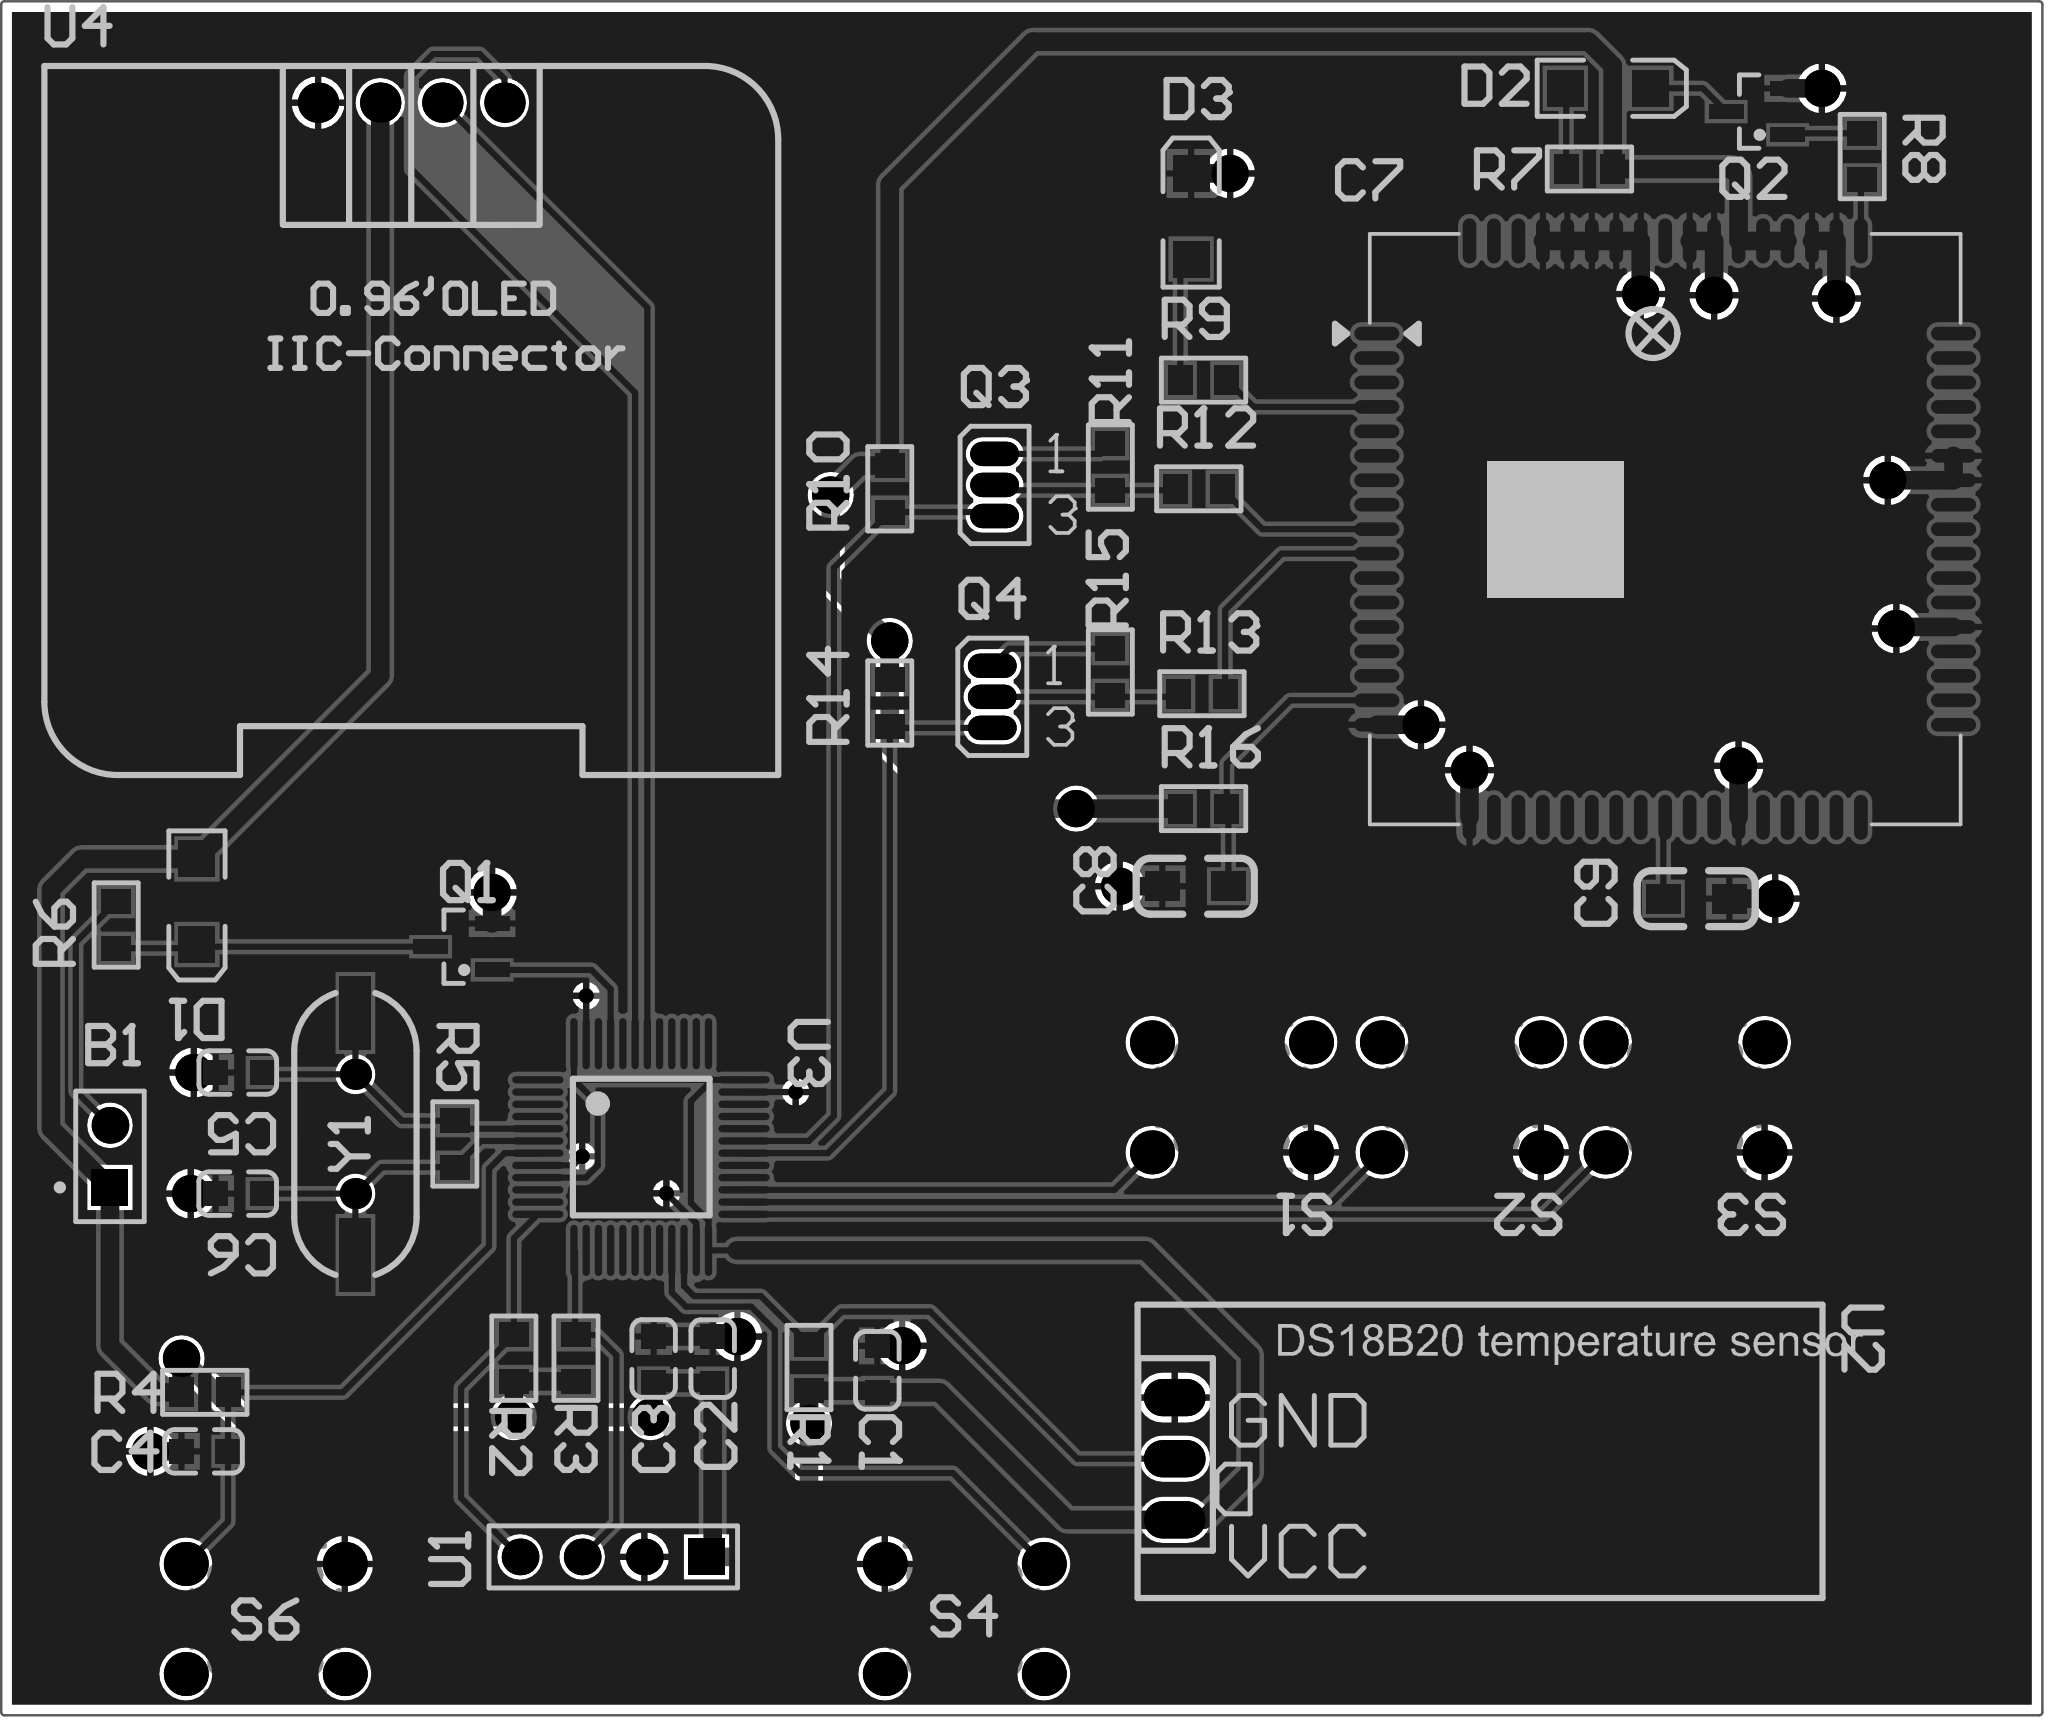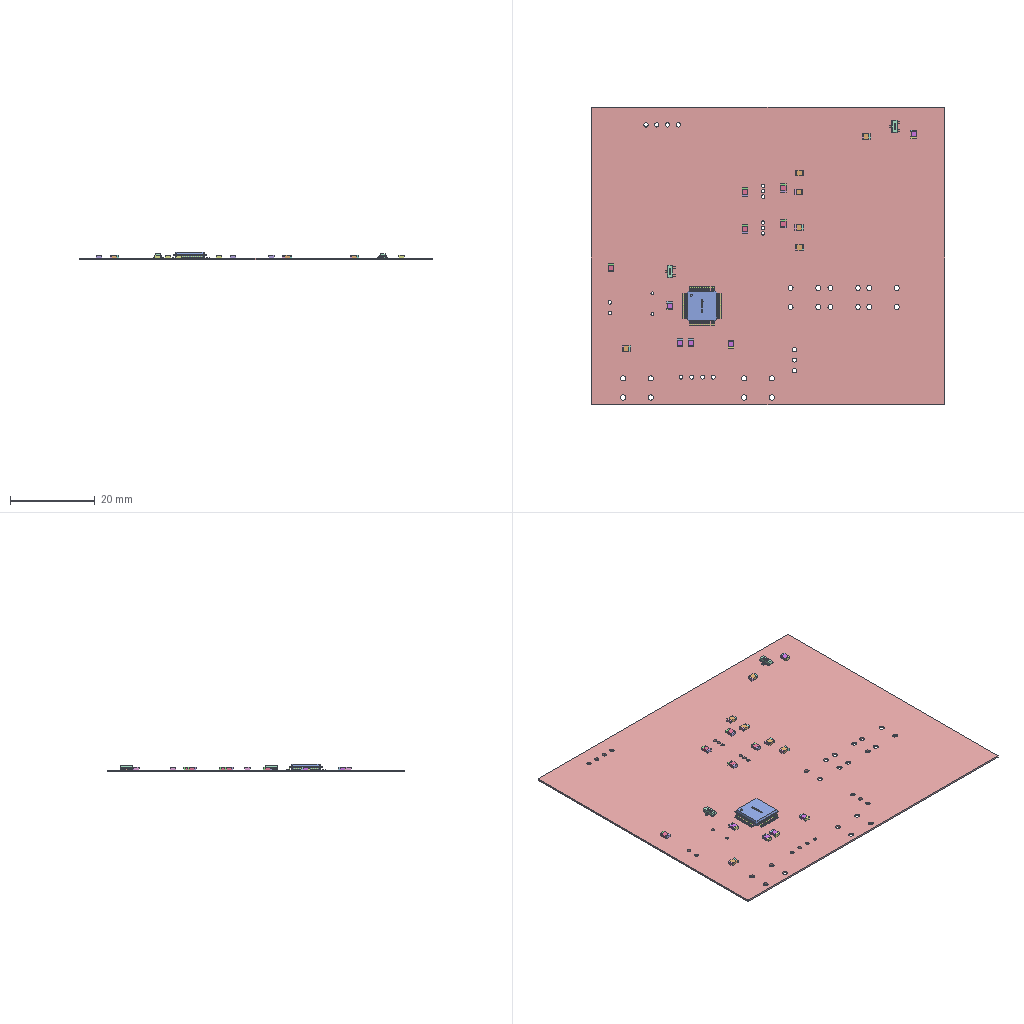Circuit board layout | Altium Designer | box 83.4 x 70.1 x 1.9 mm
Layer stack:
# Altium Designer layer stack of  (unit mm; dielectric type: 0 none, 1 core, 2 prepreg, 3 surface material)
index,name,kind,layer,copper_thickness_mm,dielectric_type,dielectric_thickness_mm,dielectric_material,dielectric_constant
0,Top Paste,other,,,,,,
1,Top Overlay,other,,,,,,
2,Top Solder,dielectric,,,3,0.0102,Solder Resist,3.5
3,Top Layer,copper,Top Layer,0.0356,,,,
4,Dielectric 1,dielectric,,,0,0.32,FR-4,4.8
5,Bottom Layer,copper,Bottom Layer,0.0356,,,,
6,Bottom Solder,dielectric,,,3,0.0102,Solder Resist,3.5
7,Bottom Overlay,other,,,,,,
8,Bottom Paste,other,,,,,,
# drill layer pairs: low layer,high layer
drill_pair,Top Layer,Bottom Layer
Part placement:
Designator,Comment,Layer,Footprint,Center-X(mm),Center-Y(mm),Rotation
Y1,XTAL,TopLayer,XTAL_US,53.086,49.049,90
U4,OLED display,TopLayer,0.96OLED_4P,55.371,91.231,360
U3,STM32,TopLayer,LQFP48_7X7,64.757,48.514,270
U2,DS18B20 temperature sensor,TopLayer,DS18B20,86.58,35.766,360
U1,ASR01 speech recognition module,TopLayer,HDR1X4,63.627,31.75,180
S6,Key,TopLayer,四脚轻触开关,49.403,29.21,0
S4,Value increase key,TopLayer,四脚轻触开关,77.978,29.21,0
S3,Value decrease key,TopLayer,四脚轻触开关,107.442,50.546,180
S2,Cursor switch key,TopLayer,四脚轻触开关,98.298,50.546,180
S1,Screen switch key,TopLayer,四脚轻触开关,88.9,50.546,180
R16,Resistor,TopLayer,0805R,87.757,62.357,0
R15,Resistor,TopLayer,0805R,83.947,67.945,90
R14,Resistor,TopLayer,0805R,74.93,66.675,90
R13,Resistor,TopLayer,0805R,87.691,67.056,0
R12,Resistor,TopLayer,0805R,87.564,75.438,0
R11,Resistor,TopLayer,0805R,83.947,76.327,90
R10,Resistor,TopLayer,0805R,74.93,75.438,90
R9,Resistor,TopLayer,0805R,87.757,79.883,0
R8,Resistor,TopLayer,0805R,114.681,89.027,270
R7,Resistor,TopLayer,0805R,103.533,88.519,0
R6,Resistor,TopLayer,0805R,43.307,57.597,90
R5,Res Semi,TopLayer,0805R,57.15,48.641,270
R4,Res Semi,TopLayer,0805R,46.929,38.481,0
R3,Resistor,TopLayer,0805R,62.103,39.878,270
R2,Resistor,TopLayer,0805R,59.563,39.878,270
R1,Resistor,TopLayer,0805R,71.628,39.497,270
Q4,MOSFET P,TopLayer,E3,79.121,66.929,0
Q3,MOSFET P,TopLayer,E3,79.216,75.595,0
Q2,N-MOSFET,TopLayer,SOT23,110.376,90.866,90
Q1,N-MOSFET,TopLayer,SOT23,57.417,56.708,90
D3,LED,TopLayer,3.2X1.6X1.1,87.249,86.586,90
D2,LED,TopLayer,3.2X1.6X1.1,104.295,91.821,360
D1,LED,TopLayer,3.2X1.6X1.1,46.609,58.547,270
C9,Capacitor,TopLayer,0805C,107.903,58.674,180
C8,Capacitor,TopLayer,0805C,87.423,59.182,180
C7,SIM800C GSM module,TopLayer,GSMM_SMD_SIM900A,106.629,73.787,0
C6,Cap,TopLayer,0603C,48.321,46.609,180
C5,Cap,TopLayer,0603C,48.326,51.562,180
C4,10uF,TopLayer,0603C,46.924,36.068,180
C3,Capacitor,TopLayer,0603C,65.278,39.817,90
C2,Capacitor,TopLayer,0603C,67.691,39.812,90
C1,Capacitor,TopLayer,0603C,74.422,39.431,270
B1,Buzzer,TopLayer,PIN2,43.053,48.133,90
Pad and via stacks:
# Altium Designer via and pad stacks of  (unit mm). Each distinct definition once, with the count of objects using it.
# via: kind,start_layer,end_layer,hole_mm,diameter_mm,mode(0 simple;1 top-mid-bottom;2 full stack),diameter_per_layer,count,example_net
# pad: kind,layer,hole_mm,hole_type(0 round;1 square;2 slot),plating,top_size,top_shape(1 round;2 rect;3 octagon;9 rounded rect),mid_size,bottom_size,mode,footprint,size_per_layer,count,example
pad,Multi-Layer,0.9,0,plated,1.5x1.5,1,1.5x1.5,1.5x1.5,0,HDR1X4,,3,U1.4
pad,Multi-Layer,0.9,0,plated,1.5x1.5,2,1.5x1.5,1.5x1.5,0,HDR1X4,,1,U1.1
pad,Multi-Layer,0.9,2,plated,2.524x1.524,1,2.524x1.524,2.524x1.524,0,DS18B20,,3,U2.2
pad,Multi-Layer,0.7112,0,plated,1.27x1.27,1,1.27x1.27,1.27x1.27,0,XTAL_US,,2,Y1.2
pad,Multi-Layer,1.2,0,plated,1.8x1.8,1,1.8x1.8,1.8x1.8,0,\u00CB\u00C4\u00BD\u00C5\u00C7\u00E1\u00B4\u00A5\u00BF\u00AA\u00B9\u00D8,,20,S6.4
pad,Multi-Layer,0.9,0,plated,1.5x1.5,2,1.5x1.5,1.5x1.5,0,PIN2,,1,B1.1
pad,Multi-Layer,0.9,0,plated,1.5x1.5,1,1.5x1.5,1.5x1.5,0,PIN2,,1,B1.2
pad,Multi-Layer,1,2,plated,1.65x1.65,1,1.65x1.65,1.65x1.65,0,0.96OLED_4P,,4,U4.1
pad,Multi-Layer,0.8,0,plated,2x1,1,2x1,2x1,0,E3,,6,Q3.1
pad,Top Layer,0,0,plated,1x1.2,2,1x1.2,1x1.2,0,0805R,,32,R1.1
pad,Top Layer,0,0,plated,1x1,2,1x1,1x1,0,0603C,,12,C1.1
pad,Top Layer,0,0,plated,0.3x2.1,1,0.3x2.1,0.3x2.1,0,LQFP48 7X7,,48,U3.48
pad,Top Layer,0,0,plated,3x1.27,2,3x1.27,3x1.27,0,XTAL_US,,2,Y1.2
pad,Top Layer,0,0,plated,1.5x1.5,2,1.5x1.5,1.5x1.5,0,3.2X1.6X1.1,,6,D1.1
pad,Top Layer,0,0,plated,0.6x1.4,2,0.6x1.4,0.6x1.4,0,SOT23,,6,Q1.D
pad,Top Layer,0,0,plated,1.85x0.56,1,1.85x0.56,1.85x0.56,0,GSMM_SMD_SIM900A,,34,C7.1
pad,Top Layer,0,0,plated,0.56x1.85,1,0.56x1.85,0.56x1.85,0,GSMM_SMD_SIM900A,,34,C7.18
pad,Top Layer,0,0,plated,1.4x1.2,2,1.4x1.2,1.4x1.2,0,0805C,,4,C8.1
via,Top Layer,Bottom Layer,0.3048,0.6096,0,,4,GND
via,Top Layer,Bottom Layer,0.762,1.524,0,,25,GND
Copper pours:
name,layer,net,type(0 solid;1 hatched;2 none)
G,Top Layer,GND,0
G,Bottom Layer,GND,0
Design rules, without the lines most boards share:
# Altium Designer design rules of  (exported by Altium Designer, unit mm)
# columns: name | kind | enabled | priority | scope1 | scope2 | descriptor | typed fields (field=value)
SilkToSilkClearance | 55 | enabled | 1 | All | All | Silk to Silk (Clearance=0mil) (All),(All) |
SilkToSolderMaskClearance | 54 | enabled | 1 | IsPad | All | Silk To Solder Mask (Clearance=0mil) (IsPad),(All) |
MinimumSolderMaskSliver | 53 | enabled | 1 | All | All | Minimum Solder Mask Sliver (Gap=0mil) (All),(All) |
HoleToHoleClearance | 52 | enabled | 1 | All | All | Hole To Hole Clearance (Gap=10mil) (All),(All) | gap=0.254
DiffPairsRouting | 51 | enabled | 1 | All | All | Differential Pairs Uncoupled Length using the Gap Constraints (Min=10mil) (Max=10mil) (Prefered=10mil)  and Width Constraints (Min=15mil) (Max=15mil) (Prefered=15mil) (All) |
SolderMaskExpansion | 13 | enabled | 1 | All | All | Solder Mask Expansion (Expansion =4mil) (All) | expansion=0.1016
PasteMaskExpansion | 14 | enabled | 1 | All | All | Paste Mask Expansion (Expansion =0mil) (All) | expansion=0
RoutingVias | 11 | enabled | 1 | All | All | Routing Via (MinHoleWidth=28mil) (MaxHoleWidth=28mil) (PreferredHoleWidth=28mil) (MinWidth=50mil) (MaxWidth=50mil) (PreferedWidth=50mil) (All) | via_min_hole=0.7112 via_max_hole=0.7112 via_preferred_diameter=1.27 via_preferred_hole=0.7112
Width | 2 | enabled | 1 | All | All | Width Constraint (Min=10mil) (Max=30mil) (Preferred=10mil) (All) |
PolygonConnect | 20 | enabled | 1 | All | All | Polygon Connect Rule(Relief Connect )(Conductor Width=10mil) (Relief Angle=90 Angle) (Entries=4) (Air Gap Width=10mil) (All),(All) | connect_style(0=relief,1=direct,2=none)=0 relief_conductor_width=0.254 relief_entries=4
PlaneConnect | 6 | enabled | 1 | All | All | Power Plane Connect Rule(Relief Connect )(Expansion=20mil) (Conductor Width=10mil) (Air Gap=10mil) (Entries=4) (All) | relief_conductor_width=0.254 relief_entries=4 relief_expansion=0.508
Clearance | 0 | enabled | 1 | All | All | Clearance Constraint (Gap=7mil) (All),(All) | gap=0.1778
Classes set for this board:
# Altium Designer classes of  (member kind: 0 net, 1 component, 2 from-to, 3 pad, 4 layer, 5 differential pair, 6 design channel, 7 polygon, 8 structure, 9 xSignal)
# columns: class name | member kind | superclass | members
12345678 | 1 | no | B1; C1; C2; C3; C4; C5; C6; C7; C8; C9; D1; D2; D3; Q1; Q2; Q3; Q4; R1; R2; R3; R4; R5; R6; R7; R8; R9; R10; R11; R12; R13; R14; R15; R16; S1; S2; S3; S4; S6; U1; U2; U3; U4; Y1;